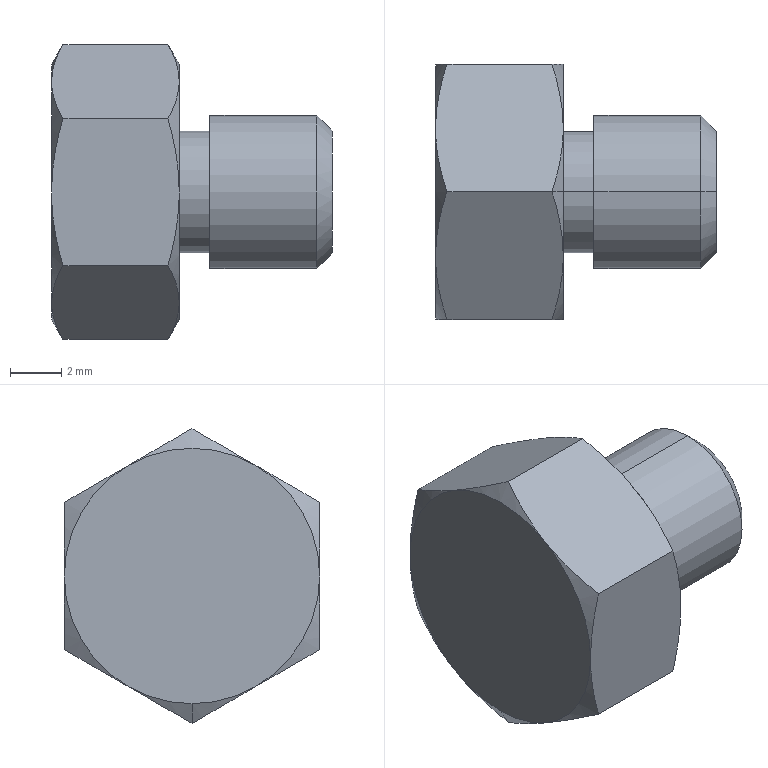Part | STEP file | 11-STEHN1011 | 1 solid | 30 faces | box 11 x 10 x 11.547 mm | volume 584.701 mm3 | cone 16 | plane 10 | cylinder 4 | commonest cylinder face diameters 4.773 x2 6 x2
STEP:
#1=CARTESIAN_POINT('',(5.386,0.,3.));
#2=VERTEX_POINT('',#1);
#3=CARTESIAN_POINT('',(5.386,0.,-3.));
#4=VERTEX_POINT('',#3);
#5=CARTESIAN_POINT('',(5.386,0.,0.));
#6=DIRECTION('',(-1.,0.,0.));
#7=DIRECTION('',(0.,0.,1.));
#8=AXIS2_PLACEMENT_3D('',#5,#6,#7);
#9=CIRCLE('',#8,3.);
#10=EDGE_CURVE('',#2,#4,#9,.T.);
#11=ORIENTED_EDGE('',*,*,#10,.T.);
#12=CARTESIAN_POINT('',(1.2,0.,-3.));
#13=VERTEX_POINT('',#12);
#14=CARTESIAN_POINT('',(5.386,0.,-3.));
#15=DIRECTION('',(-1.,0.,0.));
#16=VECTOR('',#15,1000.);
#17=LINE('',#14,#16);
#18=EDGE_CURVE('',#4,#13,#17,.T.);
#19=ORIENTED_EDGE('',*,*,#18,.T.);
#20=CARTESIAN_POINT('',(1.2,0.,3.));
#21=VERTEX_POINT('',#20);
#22=CARTESIAN_POINT('',(1.2,0.,0.));
#23=DIRECTION('',(1.,0.,0.));
#24=DIRECTION('',(0.,0.,1.));
#25=AXIS2_PLACEMENT_3D('',#22,#23,#24);
#26=CIRCLE('',#25,3.);
#27=EDGE_CURVE('',#13,#21,#26,.T.);
#28=ORIENTED_EDGE('',*,*,#27,.T.);
#29=CARTESIAN_POINT('',(5.386,0.,3.));
#30=DIRECTION('',(-1.,0.,0.));
#31=VECTOR('',#30,1000.);
#32=LINE('',#29,#31);
#33=EDGE_CURVE('',#2,#21,#32,.T.);
#34=ORIENTED_EDGE('',*,*,#33,.F.);
#35=EDGE_LOOP('',(#11,#19,#28,#34));
#36=FACE_OUTER_BOUND('',#35,.T.);
#37=CARTESIAN_POINT('',(5.386,0.,0.));
#38=DIRECTION('',(-1.,0.,0.));
#39=DIRECTION('',(0.,0.,1.));
#40=AXIS2_PLACEMENT_3D('',#37,#38,#39);
#41=CYLINDRICAL_SURFACE('',#40,3.);
#42=ADVANCED_FACE('',(#36),#41,.T.);
#43=CARTESIAN_POINT('',(6.,0.,2.386));
#44=VERTEX_POINT('',#43);
#45=CARTESIAN_POINT('',(6.,0.,-2.386));
#46=VERTEX_POINT('',#45);
#47=CARTESIAN_POINT('',(6.,0.,0.));
#48=DIRECTION('',(-1.,0.,0.));
#49=DIRECTION('',(0.,0.,1.));
#50=AXIS2_PLACEMENT_3D('',#47,#48,#49);
#51=CIRCLE('',#50,2.386);
#52=EDGE_CURVE('',#44,#46,#51,.T.);
#53=ORIENTED_EDGE('',*,*,#52,.T.);
#54=CARTESIAN_POINT('',(6.,0.,-2.386));
#55=DIRECTION('',(-0.7071,0.,-0.7071));
#56=VECTOR('',#55,1000.);
#57=LINE('',#54,#56);
#58=EDGE_CURVE('',#46,#4,#57,.T.);
#59=ORIENTED_EDGE('',*,*,#58,.T.);
#60=ORIENTED_EDGE('',*,*,#10,.F.);
#61=CARTESIAN_POINT('',(6.,0.,2.386));
#62=DIRECTION('',(-0.7071,0.,0.7071));
#63=VECTOR('',#62,1000.);
#64=LINE('',#61,#63);
#65=EDGE_CURVE('',#44,#2,#64,.T.);
#66=ORIENTED_EDGE('',*,*,#65,.F.);
#67=EDGE_LOOP('',(#53,#59,#60,#66));
#68=FACE_OUTER_BOUND('',#67,.T.);
#69=CARTESIAN_POINT('',(6.,0.,0.));
#70=DIRECTION('',(-1.,0.,0.));
#71=DIRECTION('',(0.,0.,1.));
#72=AXIS2_PLACEMENT_3D('',#69,#70,#71);
#73=CONICAL_SURFACE('',#72,2.386,0.7854);
#74=ADVANCED_FACE('',(#68),#73,.T.);
#75=CARTESIAN_POINT('',(0.,0.,-2.387));
#76=VERTEX_POINT('',#75);
#77=CARTESIAN_POINT('',(0.,0.,2.387));
#78=VERTEX_POINT('',#77);
#79=CARTESIAN_POINT('',(0.,0.,0.));
#80=DIRECTION('',(1.,0.,0.));
#81=DIRECTION('',(0.,0.,-1.));
#82=AXIS2_PLACEMENT_3D('',#79,#80,#81);
#83=CIRCLE('',#82,2.387);
#84=EDGE_CURVE('',#76,#78,#83,.T.);
#85=ORIENTED_EDGE('',*,*,#84,.T.);
#86=CARTESIAN_POINT('',(1.2,0.,2.387));
#87=VERTEX_POINT('',#86);
#88=CARTESIAN_POINT('',(0.,0.,2.387));
#89=DIRECTION('',(1.,0.,0.));
#90=VECTOR('',#89,1000.);
#91=LINE('',#88,#90);
#92=EDGE_CURVE('',#78,#87,#91,.T.);
#93=ORIENTED_EDGE('',*,*,#92,.T.);
#94=CARTESIAN_POINT('',(1.2,0.,-2.387));
#95=VERTEX_POINT('',#94);
#96=CARTESIAN_POINT('',(1.2,0.,0.));
#97=DIRECTION('',(1.,0.,0.));
#98=DIRECTION('',(0.,0.,-1.));
#99=AXIS2_PLACEMENT_3D('',#96,#97,#98);
#100=CIRCLE('',#99,2.387);
#101=EDGE_CURVE('',#95,#87,#100,.T.);
#102=ORIENTED_EDGE('',*,*,#101,.F.);
#103=CARTESIAN_POINT('',(0.,0.,-2.387));
#104=DIRECTION('',(1.,0.,0.));
#105=VECTOR('',#104,1000.);
#106=LINE('',#103,#105);
#107=EDGE_CURVE('',#76,#95,#106,.T.);
#108=ORIENTED_EDGE('',*,*,#107,.F.);
#109=EDGE_LOOP('',(#85,#93,#102,#108));
#110=FACE_OUTER_BOUND('',#109,.T.);
#111=CARTESIAN_POINT('',(0.,0.,0.));
#112=DIRECTION('',(1.,0.,0.));
#113=DIRECTION('',(0.,0.,-1.));
#114=AXIS2_PLACEMENT_3D('',#111,#112,#113);
#115=CYLINDRICAL_SURFACE('',#114,2.387);
#116=ADVANCED_FACE('',(#110),#115,.T.);
#117=CARTESIAN_POINT('',(0.,0.,5.));
#118=VERTEX_POINT('',#117);
#119=CARTESIAN_POINT('',(0.,-2.5,4.33));
#120=VERTEX_POINT('',#119);
#121=CARTESIAN_POINT('',(0.,0.,0.));
#122=DIRECTION('',(1.,0.,0.));
#123=DIRECTION('',(0.,0.,1.));
#124=AXIS2_PLACEMENT_3D('',#121,#122,#123);
#125=CIRCLE('',#124,5.);
#126=EDGE_CURVE('',#118,#120,#125,.T.);
#127=ORIENTED_EDGE('',*,*,#126,.F.);
#128=CARTESIAN_POINT('',(-0.4466,0.,5.774));
#129=VERTEX_POINT('',#128);
#130=CARTESIAN_POINT('',(0.,0.,5.));
#131=DIRECTION('',(-0.5,0.,0.866));
#132=VECTOR('',#131,1000.);
#133=LINE('',#130,#132);
#134=EDGE_CURVE('',#118,#129,#133,.T.);
#135=ORIENTED_EDGE('',*,*,#134,.T.);
#136=CARTESIAN_POINT('',(-0.4466,0.,5.774));
#137=CARTESIAN_POINT('',(-0.1743,-0.8168,5.302));
#138=CARTESIAN_POINT('',(0.,-1.647,4.823));
#139=CARTESIAN_POINT('',(0.,-2.5,4.33));
#140=B_SPLINE_CURVE_WITH_KNOTS('',3,(#136,#137,#138,#139),.UNSPECIFIED.,.F.,.F.,(4,4),(0.,0.002921),.UNSPECIFIED.);
#141=EDGE_CURVE('',#129,#120,#140,.T.);
#142=ORIENTED_EDGE('',*,*,#141,.T.);
#143=EDGE_LOOP('',(#127,#135,#142));
#144=FACE_OUTER_BOUND('',#143,.T.);
#145=CARTESIAN_POINT('',(0.,0.,0.));
#146=DIRECTION('',(-1.,0.,0.));
#147=DIRECTION('',(0.,0.,1.));
#148=AXIS2_PLACEMENT_3D('',#145,#146,#147);
#149=CONICAL_SURFACE('',#148,5.,1.047);
#150=ADVANCED_FACE('',(#144),#149,.T.);
#151=CARTESIAN_POINT('',(-5.,-2.5,-4.33));
#152=VERTEX_POINT('',#151);
#153=CARTESIAN_POINT('',(-5.,0.,-5.));
#154=VERTEX_POINT('',#153);
#155=CARTESIAN_POINT('',(-5.,0.,0.));
#156=DIRECTION('',(1.,0.,0.));
#157=DIRECTION('',(0.,0.,-1.));
#158=AXIS2_PLACEMENT_3D('',#155,#156,#157);
#159=CIRCLE('',#158,5.);
#160=EDGE_CURVE('',#152,#154,#159,.T.);
#161=ORIENTED_EDGE('',*,*,#160,.T.);
#162=CARTESIAN_POINT('',(-4.553,0.,-5.774));
#163=VERTEX_POINT('',#162);
#164=CARTESIAN_POINT('',(-5.,0.,-5.));
#165=DIRECTION('',(0.5,0.,-0.866));
#166=VECTOR('',#165,1000.);
#167=LINE('',#164,#166);
#168=EDGE_CURVE('',#154,#163,#167,.T.);
#169=ORIENTED_EDGE('',*,*,#168,.T.);
#170=CARTESIAN_POINT('',(-5.,-2.5,-4.33));
#171=CARTESIAN_POINT('',(-5.,-2.076,-4.575));
#172=CARTESIAN_POINT('',(-4.958,-1.654,-4.818));
#173=CARTESIAN_POINT('',(-4.802,-0.8183,-5.301));
#174=CARTESIAN_POINT('',(-4.689,-0.4069,-5.539));
#175=CARTESIAN_POINT('',(-4.553,0.,-5.774));
#176=B_SPLINE_CURVE_WITH_KNOTS('',3,(#170,#171,#172,#173,#174,#175),.UNSPECIFIED.,.F.,.F.,(4,2,4),(0.,0.001464,0.002928),.UNSPECIFIED.);
#177=EDGE_CURVE('',#152,#163,#176,.T.);
#178=ORIENTED_EDGE('',*,*,#177,.F.);
#179=EDGE_LOOP('',(#161,#169,#178));
#180=FACE_OUTER_BOUND('',#179,.T.);
#181=CARTESIAN_POINT('',(-5.,0.,0.));
#182=DIRECTION('',(1.,0.,0.));
#183=DIRECTION('',(0.,0.,-1.));
#184=AXIS2_PLACEMENT_3D('',#181,#182,#183);
#185=CONICAL_SURFACE('',#184,5.,1.047);
#186=ADVANCED_FACE('',(#180),#185,.T.);
#187=ORIENTED_EDGE('',*,*,#18,.F.);
#188=CARTESIAN_POINT('',(5.386,0.,0.));
#189=DIRECTION('',(-1.,0.,0.));
#190=DIRECTION('',(0.,0.,1.));
#191=AXIS2_PLACEMENT_3D('',#188,#189,#190);
#192=CIRCLE('',#191,3.);
#193=EDGE_CURVE('',#4,#2,#192,.T.);
#194=ORIENTED_EDGE('',*,*,#193,.T.);
#195=ORIENTED_EDGE('',*,*,#33,.T.);
#196=CARTESIAN_POINT('',(1.2,0.,0.));
#197=DIRECTION('',(1.,0.,0.));
#198=DIRECTION('',(0.,0.,1.));
#199=AXIS2_PLACEMENT_3D('',#196,#197,#198);
#200=CIRCLE('',#199,3.);
#201=EDGE_CURVE('',#21,#13,#200,.T.);
#202=ORIENTED_EDGE('',*,*,#201,.T.);
#203=EDGE_LOOP('',(#187,#194,#195,#202));
#204=FACE_OUTER_BOUND('',#203,.T.);
#205=CARTESIAN_POINT('',(5.386,0.,0.));
#206=DIRECTION('',(-1.,0.,0.));
#207=DIRECTION('',(0.,0.,1.));
#208=AXIS2_PLACEMENT_3D('',#205,#206,#207);
#209=CYLINDRICAL_SURFACE('',#208,3.);
#210=ADVANCED_FACE('',(#204),#209,.T.);
#211=ORIENTED_EDGE('',*,*,#58,.F.);
#212=CARTESIAN_POINT('',(6.,0.,0.));
#213=DIRECTION('',(-1.,0.,0.));
#214=DIRECTION('',(0.,0.,1.));
#215=AXIS2_PLACEMENT_3D('',#212,#213,#214);
#216=CIRCLE('',#215,2.386);
#217=EDGE_CURVE('',#46,#44,#216,.T.);
#218=ORIENTED_EDGE('',*,*,#217,.T.);
#219=ORIENTED_EDGE('',*,*,#65,.T.);
#220=ORIENTED_EDGE('',*,*,#193,.F.);
#221=EDGE_LOOP('',(#211,#218,#219,#220));
#222=FACE_OUTER_BOUND('',#221,.T.);
#223=CARTESIAN_POINT('',(6.,0.,0.));
#224=DIRECTION('',(-1.,0.,0.));
#225=DIRECTION('',(0.,0.,1.));
#226=AXIS2_PLACEMENT_3D('',#223,#224,#225);
#227=CONICAL_SURFACE('',#226,2.386,0.7854);
#228=ADVANCED_FACE('',(#222),#227,.T.);
#229=ORIENTED_EDGE('',*,*,#101,.T.);
#230=CARTESIAN_POINT('',(1.2,0.,0.));
#231=DIRECTION('',(1.,0.,0.));
#232=DIRECTION('',(0.,0.,-1.));
#233=AXIS2_PLACEMENT_3D('',#230,#231,#232);
#234=CIRCLE('',#233,2.387);
#235=EDGE_CURVE('',#87,#95,#234,.T.);
#236=ORIENTED_EDGE('',*,*,#235,.T.);
#237=EDGE_LOOP('',(#229,#236));
#238=FACE_BOUND('',#237,.T.);
#239=ORIENTED_EDGE('',*,*,#201,.F.);
#240=ORIENTED_EDGE('',*,*,#27,.F.);
#241=EDGE_LOOP('',(#239,#240));
#242=FACE_OUTER_BOUND('',#241,.T.);
#243=CARTESIAN_POINT('',(1.2,3.,3.));
#244=DIRECTION('',(-1.,0.,0.));
#245=DIRECTION('',(0.,0.,-1.));
#246=AXIS2_PLACEMENT_3D('',#243,#244,#245);
#247=PLANE('',#246);
#248=ADVANCED_FACE('',(#238,#242),#247,.T.);
#249=ORIENTED_EDGE('',*,*,#52,.F.);
#250=ORIENTED_EDGE('',*,*,#217,.F.);
#251=EDGE_LOOP('',(#249,#250));
#252=FACE_OUTER_BOUND('',#251,.T.);
#253=CARTESIAN_POINT('',(6.,2.386,-2.386));
#254=DIRECTION('',(1.,0.,0.));
#255=DIRECTION('',(0.,0.,1.));
#256=AXIS2_PLACEMENT_3D('',#253,#254,#255);
#257=PLANE('',#256);
#258=ADVANCED_FACE('',(#252),#257,.T.);
#259=ORIENTED_EDGE('',*,*,#92,.F.);
#260=CARTESIAN_POINT('',(0.,0.,0.));
#261=DIRECTION('',(1.,0.,0.));
#262=DIRECTION('',(0.,0.,-1.));
#263=AXIS2_PLACEMENT_3D('',#260,#261,#262);
#264=CIRCLE('',#263,2.387);
#265=EDGE_CURVE('',#78,#76,#264,.T.);
#266=ORIENTED_EDGE('',*,*,#265,.T.);
#267=ORIENTED_EDGE('',*,*,#107,.T.);
#268=ORIENTED_EDGE('',*,*,#235,.F.);
#269=EDGE_LOOP('',(#259,#266,#267,#268));
#270=FACE_OUTER_BOUND('',#269,.T.);
#271=CARTESIAN_POINT('',(0.,0.,0.));
#272=DIRECTION('',(1.,0.,0.));
#273=DIRECTION('',(0.,0.,-1.));
#274=AXIS2_PLACEMENT_3D('',#271,#272,#273);
#275=CYLINDRICAL_SURFACE('',#274,2.387);
#276=ADVANCED_FACE('',(#270),#275,.T.);
#277=ORIENTED_EDGE('',*,*,#84,.F.);
#278=ORIENTED_EDGE('',*,*,#265,.F.);
#279=EDGE_LOOP('',(#277,#278));
#280=FACE_BOUND('',#279,.T.);
#281=CARTESIAN_POINT('',(0.,-5.,0.));
#282=VERTEX_POINT('',#281);
#283=CARTESIAN_POINT('',(0.,0.,0.));
#284=DIRECTION('',(1.,0.,0.));
#285=DIRECTION('',(0.,0.,1.));
#286=AXIS2_PLACEMENT_3D('',#283,#284,#285);
#287=CIRCLE('',#286,5.);
#288=EDGE_CURVE('',#120,#282,#287,.T.);
#289=ORIENTED_EDGE('',*,*,#288,.T.);
#290=CARTESIAN_POINT('',(0.,-2.5,-4.33));
#291=VERTEX_POINT('',#290);
#292=CARTESIAN_POINT('',(0.,0.,0.));
#293=DIRECTION('',(1.,0.,0.));
#294=DIRECTION('',(0.,0.,1.));
#295=AXIS2_PLACEMENT_3D('',#292,#293,#294);
#296=CIRCLE('',#295,5.);
#297=EDGE_CURVE('',#282,#291,#296,.T.);
#298=ORIENTED_EDGE('',*,*,#297,.T.);
#299=CARTESIAN_POINT('',(0.,2.5,-4.33));
#300=VERTEX_POINT('',#299);
#301=CARTESIAN_POINT('',(0.,0.,0.));
#302=DIRECTION('',(1.,0.,0.));
#303=DIRECTION('',(0.,0.,1.));
#304=AXIS2_PLACEMENT_3D('',#301,#302,#303);
#305=CIRCLE('',#304,5.);
#306=EDGE_CURVE('',#291,#300,#305,.T.);
#307=ORIENTED_EDGE('',*,*,#306,.T.);
#308=CARTESIAN_POINT('',(0.,5.,0.));
#309=VERTEX_POINT('',#308);
#310=CARTESIAN_POINT('',(0.,0.,0.));
#311=DIRECTION('',(1.,0.,0.));
#312=DIRECTION('',(0.,0.,1.));
#313=AXIS2_PLACEMENT_3D('',#310,#311,#312);
#314=CIRCLE('',#313,5.);
#315=EDGE_CURVE('',#300,#309,#314,.T.);
#316=ORIENTED_EDGE('',*,*,#315,.T.);
#317=CARTESIAN_POINT('',(0.,2.5,4.33));
#318=VERTEX_POINT('',#317);
#319=CARTESIAN_POINT('',(0.,0.,0.));
#320=DIRECTION('',(1.,0.,0.));
#321=DIRECTION('',(0.,0.,1.));
#322=AXIS2_PLACEMENT_3D('',#319,#320,#321);
#323=CIRCLE('',#322,5.);
#324=EDGE_CURVE('',#309,#318,#323,.T.);
#325=ORIENTED_EDGE('',*,*,#324,.T.);
#326=CARTESIAN_POINT('',(0.,0.,0.));
#327=DIRECTION('',(1.,0.,0.));
#328=DIRECTION('',(0.,0.,1.));
#329=AXIS2_PLACEMENT_3D('',#326,#327,#328);
#330=CIRCLE('',#329,5.);
#331=EDGE_CURVE('',#318,#118,#330,.T.);
#332=ORIENTED_EDGE('',*,*,#331,.T.);
#333=ORIENTED_EDGE('',*,*,#126,.T.);
#334=EDGE_LOOP('',(#289,#298,#307,#316,#325,#332,#333));
#335=FACE_OUTER_BOUND('',#334,.T.);
#336=CARTESIAN_POINT('',(0.,-5.,5.));
#337=DIRECTION('',(1.,0.,0.));
#338=DIRECTION('',(0.,0.,-1.));
#339=AXIS2_PLACEMENT_3D('',#336,#337,#338);
#340=PLANE('',#339);
#341=ADVANCED_FACE('',(#280,#335),#340,.T.);
#342=CARTESIAN_POINT('',(-0.4466,-5.,-2.887));
#343=VERTEX_POINT('',#342);
#344=CARTESIAN_POINT('',(-0.4466,-5.,-2.887));
#345=CARTESIAN_POINT('',(-0.1743,-4.183,-3.358));
#346=CARTESIAN_POINT('',(0.,-3.353,-3.837));
#347=CARTESIAN_POINT('',(0.,-2.5,-4.33));
#348=B_SPLINE_CURVE_WITH_KNOTS('',3,(#344,#345,#346,#347),.UNSPECIFIED.,.F.,.F.,(4,4),(0.,0.002921),.UNSPECIFIED.);
#349=EDGE_CURVE('',#343,#291,#348,.T.);
#350=ORIENTED_EDGE('',*,*,#349,.T.);
#351=ORIENTED_EDGE('',*,*,#297,.F.);
#352=CARTESIAN_POINT('',(0.,-5.,0.));
#353=CARTESIAN_POINT('',(0.,-5.,-0.9853));
#354=CARTESIAN_POINT('',(-0.1743,-5.,-1.944));
#355=CARTESIAN_POINT('',(-0.4466,-5.,-2.887));
#356=B_SPLINE_CURVE_WITH_KNOTS('',3,(#352,#353,#354,#355),.UNSPECIFIED.,.F.,.F.,(4,4),(0.,0.002921),.UNSPECIFIED.);
#357=EDGE_CURVE('',#282,#343,#356,.T.);
#358=ORIENTED_EDGE('',*,*,#357,.T.);
#359=EDGE_LOOP('',(#350,#351,#358));
#360=FACE_OUTER_BOUND('',#359,.T.);
#361=CARTESIAN_POINT('',(0.,0.,0.));
#362=DIRECTION('',(-1.,0.,0.));
#363=DIRECTION('',(0.,0.,1.));
#364=AXIS2_PLACEMENT_3D('',#361,#362,#363);
#365=CONICAL_SURFACE('',#364,5.,1.047);
#366=ADVANCED_FACE('',(#360),#365,.T.);
#367=CARTESIAN_POINT('',(-0.4466,-5.,2.887));
#368=VERTEX_POINT('',#367);
#369=CARTESIAN_POINT('',(-0.4466,-5.,2.887));
#370=CARTESIAN_POINT('',(-0.3109,-5.,2.417));
#371=CARTESIAN_POINT('',(-0.1985,-5.,1.942));
#372=CARTESIAN_POINT('',(-0.04234,-5.,0.9764));
#373=CARTESIAN_POINT('',(0.,-5.,0.4895));
#374=CARTESIAN_POINT('',(0.,-5.,0.));
#375=B_SPLINE_CURVE_WITH_KNOTS('',3,(#369,#370,#371,#372,#373,#374),.UNSPECIFIED.,.F.,.F.,(4,2,4),(-0.00158,-0.0001154,0.001349),.UNSPECIFIED.);
#376=EDGE_CURVE('',#368,#282,#375,.T.);
#377=ORIENTED_EDGE('',*,*,#376,.T.);
#378=ORIENTED_EDGE('',*,*,#288,.F.);
#379=CARTESIAN_POINT('',(0.,-2.5,4.33));
#380=CARTESIAN_POINT('',(0.,-3.353,3.837));
#381=CARTESIAN_POINT('',(-0.1743,-4.183,3.358));
#382=CARTESIAN_POINT('',(-0.4466,-5.,2.887));
#383=B_SPLINE_CURVE_WITH_KNOTS('',3,(#379,#380,#381,#382),.UNSPECIFIED.,.F.,.F.,(4,4),(0.,0.002921),.UNSPECIFIED.);
#384=EDGE_CURVE('',#120,#368,#383,.T.);
#385=ORIENTED_EDGE('',*,*,#384,.T.);
#386=EDGE_LOOP('',(#377,#378,#385));
#387=FACE_OUTER_BOUND('',#386,.T.);
#388=CARTESIAN_POINT('',(0.,0.,0.));
#389=DIRECTION('',(-1.,0.,0.));
#390=DIRECTION('',(0.,0.,1.));
#391=AXIS2_PLACEMENT_3D('',#388,#389,#390);
#392=CONICAL_SURFACE('',#391,5.,1.047);
#393=ADVANCED_FACE('',(#387),#392,.T.);
#394=ORIENTED_EDGE('',*,*,#134,.F.);
#395=ORIENTED_EDGE('',*,*,#331,.F.);
#396=CARTESIAN_POINT('',(0.,2.5,4.33));
#397=CARTESIAN_POINT('',(0.,1.647,4.823));
#398=CARTESIAN_POINT('',(-0.1743,0.8168,5.302));
#399=CARTESIAN_POINT('',(-0.4466,0.,5.774));
#400=B_SPLINE_CURVE_WITH_KNOTS('',3,(#396,#397,#398,#399),.UNSPECIFIED.,.F.,.F.,(4,4),(0.,0.002921),.UNSPECIFIED.);
#401=EDGE_CURVE('',#318,#129,#400,.T.);
#402=ORIENTED_EDGE('',*,*,#401,.T.);
#403=EDGE_LOOP('',(#394,#395,#402));
#404=FACE_OUTER_BOUND('',#403,.T.);
#405=CARTESIAN_POINT('',(0.,0.,0.));
#406=DIRECTION('',(-1.,0.,0.));
#407=DIRECTION('',(0.,0.,1.));
#408=AXIS2_PLACEMENT_3D('',#405,#406,#407);
#409=CONICAL_SURFACE('',#408,5.,1.047);
#410=ADVANCED_FACE('',(#404),#409,.T.);
#411=ORIENTED_EDGE('',*,*,#324,.F.);
#412=CARTESIAN_POINT('',(-0.4466,5.,2.887));
#413=VERTEX_POINT('',#412);
#414=CARTESIAN_POINT('',(0.,5.,0.));
#415=CARTESIAN_POINT('',(0.,5.,0.9853));
#416=CARTESIAN_POINT('',(-0.1743,5.,1.944));
#417=CARTESIAN_POINT('',(-0.4466,5.,2.887));
#418=B_SPLINE_CURVE_WITH_KNOTS('',3,(#414,#415,#416,#417),.UNSPECIFIED.,.F.,.F.,(4,4),(0.,0.002921),.UNSPECIFIED.);
#419=EDGE_CURVE('',#309,#413,#418,.T.);
#420=ORIENTED_EDGE('',*,*,#419,.T.);
#421=CARTESIAN_POINT('',(-0.4466,5.,2.887));
#422=CARTESIAN_POINT('',(-0.1743,4.183,3.358));
#423=CARTESIAN_POINT('',(0.,3.353,3.837));
#424=CARTESIAN_POINT('',(0.,2.5,4.33));
#425=B_SPLINE_CURVE_WITH_KNOTS('',3,(#421,#422,#423,#424),.UNSPECIFIED.,.F.,.F.,(4,4),(0.,0.002921),.UNSPECIFIED.);
#426=EDGE_CURVE('',#413,#318,#425,.T.);
#427=ORIENTED_EDGE('',*,*,#426,.T.);
#428=EDGE_LOOP('',(#411,#420,#427));
#429=FACE_OUTER_BOUND('',#428,.T.);
#430=CARTESIAN_POINT('',(0.,0.,0.));
#431=DIRECTION('',(-1.,0.,0.));
#432=DIRECTION('',(0.,0.,1.));
#433=AXIS2_PLACEMENT_3D('',#430,#431,#432);
#434=CONICAL_SURFACE('',#433,5.,1.047);
#435=ADVANCED_FACE('',(#429),#434,.T.);
#436=CARTESIAN_POINT('',(-0.4466,5.,-2.887));
#437=VERTEX_POINT('',#436);
#438=CARTESIAN_POINT('',(-0.4466,5.,-2.887));
#439=CARTESIAN_POINT('',(-0.3109,5.,-2.417));
#440=CARTESIAN_POINT('',(-0.1985,5.,-1.942));
#441=CARTESIAN_POINT('',(-0.04234,5.,-0.9764));
#442=CARTESIAN_POINT('',(0.,5.,-0.4895));
#443=CARTESIAN_POINT('',(0.,5.,0.));
#444=B_SPLINE_CURVE_WITH_KNOTS('',3,(#438,#439,#440,#441,#442,#443),.UNSPECIFIED.,.F.,.F.,(4,2,4),(-0.00158,-0.0001154,0.001349),.UNSPECIFIED.);
#445=EDGE_CURVE('',#437,#309,#444,.T.);
#446=ORIENTED_EDGE('',*,*,#445,.T.);
#447=ORIENTED_EDGE('',*,*,#315,.F.);
#448=CARTESIAN_POINT('',(0.,2.5,-4.33));
#449=CARTESIAN_POINT('',(0.,3.353,-3.837));
#450=CARTESIAN_POINT('',(-0.1743,4.183,-3.358));
#451=CARTESIAN_POINT('',(-0.4466,5.,-2.887));
#452=B_SPLINE_CURVE_WITH_KNOTS('',3,(#448,#449,#450,#451),.UNSPECIFIED.,.F.,.F.,(4,4),(0.,0.002921),.UNSPECIFIED.);
#453=EDGE_CURVE('',#300,#437,#452,.T.);
#454=ORIENTED_EDGE('',*,*,#453,.T.);
#455=EDGE_LOOP('',(#446,#447,#454));
#456=FACE_OUTER_BOUND('',#455,.T.);
#457=CARTESIAN_POINT('',(0.,0.,0.));
#458=DIRECTION('',(-1.,0.,0.));
#459=DIRECTION('',(0.,0.,1.));
#460=AXIS2_PLACEMENT_3D('',#457,#458,#459);
#461=CONICAL_SURFACE('',#460,5.,1.047);
#462=ADVANCED_FACE('',(#456),#461,.T.);
#463=ORIENTED_EDGE('',*,*,#306,.F.);
#464=CARTESIAN_POINT('',(-0.4466,0.,-5.774));
#465=VERTEX_POINT('',#464);
#466=CARTESIAN_POINT('',(0.,-2.5,-4.33));
#467=CARTESIAN_POINT('',(0.,-1.647,-4.823));
#468=CARTESIAN_POINT('',(-0.1743,-0.8168,-5.302));
#469=CARTESIAN_POINT('',(-0.4466,0.,-5.774));
#470=B_SPLINE_CURVE_WITH_KNOTS('',3,(#466,#467,#468,#469),.UNSPECIFIED.,.F.,.F.,(4,4),(0.,0.002921),.UNSPECIFIED.);
#471=EDGE_CURVE('',#291,#465,#470,.T.);
#472=ORIENTED_EDGE('',*,*,#471,.T.);
#473=CARTESIAN_POINT('',(-0.4466,0.,-5.774));
#474=CARTESIAN_POINT('',(-0.1743,0.8168,-5.302));
#475=CARTESIAN_POINT('',(0.,1.647,-4.823));
#476=CARTESIAN_POINT('',(0.,2.5,-4.33));
#477=B_SPLINE_CURVE_WITH_KNOTS('',3,(#473,#474,#475,#476),.UNSPECIFIED.,.F.,.F.,(4,4),(0.,0.002921),.UNSPECIFIED.);
#478=EDGE_CURVE('',#465,#300,#477,.T.);
#479=ORIENTED_EDGE('',*,*,#478,.T.);
#480=EDGE_LOOP('',(#463,#472,#479));
#481=FACE_OUTER_BOUND('',#480,.T.);
#482=CARTESIAN_POINT('',(0.,0.,0.));
#483=DIRECTION('',(-1.,0.,0.));
#484=DIRECTION('',(0.,0.,1.));
#485=AXIS2_PLACEMENT_3D('',#482,#483,#484);
#486=CONICAL_SURFACE('',#485,5.,1.047);
#487=ADVANCED_FACE('',(#481),#486,.T.);
#488=CARTESIAN_POINT('',(-2.5,0.,-5.774));
#489=DIRECTION('',(1.,0.,0.));
#490=VECTOR('',#489,1000.);
#491=LINE('',#488,#490);
#492=EDGE_CURVE('',#163,#465,#491,.T.);
#493=ORIENTED_EDGE('',*,*,#492,.T.);
#494=ORIENTED_EDGE('',*,*,#471,.F.);
#495=ORIENTED_EDGE('',*,*,#349,.F.);
#496=CARTESIAN_POINT('',(-4.553,-5.,-2.887));
#497=VERTEX_POINT('',#496);
#498=CARTESIAN_POINT('',(-2.5,-5.,-2.887));
#499=DIRECTION('',(-1.,0.,0.));
#500=VECTOR('',#499,1000.);
#501=LINE('',#498,#500);
#502=EDGE_CURVE('',#343,#497,#501,.T.);
#503=ORIENTED_EDGE('',*,*,#502,.T.);
#504=CARTESIAN_POINT('',(-4.553,-5.,-2.887));
#505=CARTESIAN_POINT('',(-4.826,-4.183,-3.358));
#506=CARTESIAN_POINT('',(-5.,-3.353,-3.837));
#507=CARTESIAN_POINT('',(-5.,-2.5,-4.33));
#508=B_SPLINE_CURVE_WITH_KNOTS('',3,(#504,#505,#506,#507),.UNSPECIFIED.,.F.,.F.,(4,4),(0.,0.002921),.UNSPECIFIED.);
#509=EDGE_CURVE('',#497,#152,#508,.T.);
#510=ORIENTED_EDGE('',*,*,#509,.T.);
#511=ORIENTED_EDGE('',*,*,#177,.T.);
#512=EDGE_LOOP('',(#493,#494,#495,#503,#510,#511));
#513=FACE_OUTER_BOUND('',#512,.T.);
#514=CARTESIAN_POINT('',(0.,-5.,-2.887));
#515=DIRECTION('',(0.,-0.5,-0.866));
#516=DIRECTION('',(-1.,0.,0.));
#517=AXIS2_PLACEMENT_3D('',#514,#515,#516);
#518=PLANE('',#517);
#519=ADVANCED_FACE('',(#513),#518,.T.);
#520=ORIENTED_EDGE('',*,*,#502,.F.);
#521=ORIENTED_EDGE('',*,*,#357,.F.);
#522=ORIENTED_EDGE('',*,*,#376,.F.);
#523=CARTESIAN_POINT('',(-4.553,-5.,2.887));
#524=VERTEX_POINT('',#523);
#525=CARTESIAN_POINT('',(-2.5,-5.,2.887));
#526=DIRECTION('',(-1.,0.,0.));
#527=VECTOR('',#526,1000.);
#528=LINE('',#525,#527);
#529=EDGE_CURVE('',#368,#524,#528,.T.);
#530=ORIENTED_EDGE('',*,*,#529,.T.);
#531=CARTESIAN_POINT('',(-5.,-5.,0.));
#532=VERTEX_POINT('',#531);
#533=CARTESIAN_POINT('',(-4.553,-5.,2.887));
#534=CARTESIAN_POINT('',(-4.826,-5.,1.944));
#535=CARTESIAN_POINT('',(-5.,-5.,0.9853));
#536=CARTESIAN_POINT('',(-5.,-5.,0.));
#537=B_SPLINE_CURVE_WITH_KNOTS('',3,(#533,#534,#535,#536),.UNSPECIFIED.,.F.,.F.,(4,4),(0.,0.002921),.UNSPECIFIED.);
#538=EDGE_CURVE('',#524,#532,#537,.T.);
#539=ORIENTED_EDGE('',*,*,#538,.T.);
#540=CARTESIAN_POINT('',(-5.,-5.,0.));
#541=CARTESIAN_POINT('',(-5.,-5.,-0.9853));
#542=CARTESIAN_POINT('',(-4.826,-5.,-1.944));
#543=CARTESIAN_POINT('',(-4.553,-5.,-2.887));
#544=B_SPLINE_CURVE_WITH_KNOTS('',3,(#540,#541,#542,#543),.UNSPECIFIED.,.F.,.F.,(4,4),(0.,0.002921),.UNSPECIFIED.);
#545=EDGE_CURVE('',#532,#497,#544,.T.);
#546=ORIENTED_EDGE('',*,*,#545,.T.);
#547=EDGE_LOOP('',(#520,#521,#522,#530,#539,#546));
#548=FACE_OUTER_BOUND('',#547,.T.);
#549=CARTESIAN_POINT('',(-5.,-5.,-2.887));
#550=DIRECTION('',(0.,-1.,0.));
#551=DIRECTION('',(1.,0.,0.));
#552=AXIS2_PLACEMENT_3D('',#549,#550,#551);
#553=PLANE('',#552);
#554=ADVANCED_FACE('',(#548),#553,.T.);
#555=ORIENTED_EDGE('',*,*,#529,.F.);
#556=ORIENTED_EDGE('',*,*,#384,.F.);
#557=ORIENTED_EDGE('',*,*,#141,.F.);
#558=CARTESIAN_POINT('',(-4.553,0.,5.774));
#559=VERTEX_POINT('',#558);
#560=CARTESIAN_POINT('',(-2.5,0.,5.774));
#561=DIRECTION('',(-1.,0.,0.));
#562=VECTOR('',#561,1000.);
#563=LINE('',#560,#562);
#564=EDGE_CURVE('',#129,#559,#563,.T.);
#565=ORIENTED_EDGE('',*,*,#564,.T.);
#566=CARTESIAN_POINT('',(-5.,-2.5,4.33));
#567=VERTEX_POINT('',#566);
#568=CARTESIAN_POINT('',(-4.553,0.,5.774));
#569=CARTESIAN_POINT('',(-4.826,-0.8168,5.302));
#570=CARTESIAN_POINT('',(-5.,-1.647,4.823));
#571=CARTESIAN_POINT('',(-5.,-2.5,4.33));
#572=B_SPLINE_CURVE_WITH_KNOTS('',3,(#568,#569,#570,#571),.UNSPECIFIED.,.F.,.F.,(4,4),(0.,0.002921),.UNSPECIFIED.);
#573=EDGE_CURVE('',#559,#567,#572,.T.);
#574=ORIENTED_EDGE('',*,*,#573,.T.);
#575=CARTESIAN_POINT('',(-5.,-2.5,4.33));
#576=CARTESIAN_POINT('',(-5.,-3.353,3.837));
#577=CARTESIAN_POINT('',(-4.826,-4.183,3.358));
#578=CARTESIAN_POINT('',(-4.553,-5.,2.887));
#579=B_SPLINE_CURVE_WITH_KNOTS('',3,(#575,#576,#577,#578),.UNSPECIFIED.,.F.,.F.,(4,4),(0.,0.002921),.UNSPECIFIED.);
#580=EDGE_CURVE('',#567,#524,#579,.T.);
#581=ORIENTED_EDGE('',*,*,#580,.T.);
#582=EDGE_LOOP('',(#555,#556,#557,#565,#574,#581));
#583=FACE_OUTER_BOUND('',#582,.T.);
#584=CARTESIAN_POINT('',(-5.,-5.,2.887));
#585=DIRECTION('',(0.,-0.5,0.866));
#586=DIRECTION('',(1.,0.,0.));
#587=AXIS2_PLACEMENT_3D('',#584,#585,#586);
#588=PLANE('',#587);
#589=ADVANCED_FACE('',(#583),#588,.T.);
#590=CARTESIAN_POINT('',(-5.,2.5,4.33));
#591=VERTEX_POINT('',#590);
#592=CARTESIAN_POINT('',(-5.,2.5,4.33));
#593=CARTESIAN_POINT('',(-5.,2.076,4.575));
#594=CARTESIAN_POINT('',(-4.958,1.654,4.818));
#595=CARTESIAN_POINT('',(-4.802,0.8183,5.301));
#596=CARTESIAN_POINT('',(-4.689,0.4069,5.539));
#597=CARTESIAN_POINT('',(-4.553,0.,5.774));
#598=B_SPLINE_CURVE_WITH_KNOTS('',3,(#592,#593,#594,#595,#596,#597),.UNSPECIFIED.,.F.,.F.,(4,2,4),(-0.001349,0.0001154,0.00158),.UNSPECIFIED.);
#599=EDGE_CURVE('',#591,#559,#598,.T.);
#600=ORIENTED_EDGE('',*,*,#599,.T.);
#601=ORIENTED_EDGE('',*,*,#564,.F.);
#602=ORIENTED_EDGE('',*,*,#401,.F.);
#603=ORIENTED_EDGE('',*,*,#426,.F.);
#604=CARTESIAN_POINT('',(-4.553,5.,2.887));
#605=VERTEX_POINT('',#604);
#606=CARTESIAN_POINT('',(-2.5,5.,2.887));
#607=DIRECTION('',(-1.,0.,0.));
#608=VECTOR('',#607,1000.);
#609=LINE('',#606,#608);
#610=EDGE_CURVE('',#413,#605,#609,.T.);
#611=ORIENTED_EDGE('',*,*,#610,.T.);
#612=CARTESIAN_POINT('',(-4.553,5.,2.887));
#613=CARTESIAN_POINT('',(-4.826,4.183,3.358));
#614=CARTESIAN_POINT('',(-5.,3.353,3.837));
#615=CARTESIAN_POINT('',(-5.,2.5,4.33));
#616=B_SPLINE_CURVE_WITH_KNOTS('',3,(#612,#613,#614,#615),.UNSPECIFIED.,.F.,.F.,(4,4),(0.,0.002921),.UNSPECIFIED.);
#617=EDGE_CURVE('',#605,#591,#616,.T.);
#618=ORIENTED_EDGE('',*,*,#617,.T.);
#619=EDGE_LOOP('',(#600,#601,#602,#603,#611,#618));
#620=FACE_OUTER_BOUND('',#619,.T.);
#621=CARTESIAN_POINT('',(-5.,0.,5.774));
#622=DIRECTION('',(0.,0.5,0.866));
#623=DIRECTION('',(1.,0.,0.));
#624=AXIS2_PLACEMENT_3D('',#621,#622,#623);
#625=PLANE('',#624);
#626=ADVANCED_FACE('',(#620),#625,.T.);
#627=CARTESIAN_POINT('',(-5.,5.,0.));
#628=VERTEX_POINT('',#627);
#629=CARTESIAN_POINT('',(-5.,5.,0.));
#630=CARTESIAN_POINT('',(-5.,5.,0.9853));
#631=CARTESIAN_POINT('',(-4.826,5.,1.944));
#632=CARTESIAN_POINT('',(-4.553,5.,2.887));
#633=B_SPLINE_CURVE_WITH_KNOTS('',3,(#629,#630,#631,#632),.UNSPECIFIED.,.F.,.F.,(4,4),(0.,0.002921),.UNSPECIFIED.);
#634=EDGE_CURVE('',#628,#605,#633,.T.);
#635=ORIENTED_EDGE('',*,*,#634,.T.);
#636=ORIENTED_EDGE('',*,*,#610,.F.);
#637=ORIENTED_EDGE('',*,*,#419,.F.);
#638=ORIENTED_EDGE('',*,*,#445,.F.);
#639=CARTESIAN_POINT('',(-4.553,5.,-2.887));
#640=VERTEX_POINT('',#639);
#641=CARTESIAN_POINT('',(-2.5,5.,-2.887));
#642=DIRECTION('',(-1.,0.,0.));
#643=VECTOR('',#642,1000.);
#644=LINE('',#641,#643);
#645=EDGE_CURVE('',#437,#640,#644,.T.);
#646=ORIENTED_EDGE('',*,*,#645,.T.);
#647=CARTESIAN_POINT('',(-4.553,5.,-2.887));
#648=CARTESIAN_POINT('',(-4.826,5.,-1.944));
#649=CARTESIAN_POINT('',(-5.,5.,-0.9853));
#650=CARTESIAN_POINT('',(-5.,5.,0.));
#651=B_SPLINE_CURVE_WITH_KNOTS('',3,(#647,#648,#649,#650),.UNSPECIFIED.,.F.,.F.,(4,4),(0.,0.002921),.UNSPECIFIED.);
#652=EDGE_CURVE('',#640,#628,#651,.T.);
#653=ORIENTED_EDGE('',*,*,#652,.T.);
#654=EDGE_LOOP('',(#635,#636,#637,#638,#646,#653));
#655=FACE_OUTER_BOUND('',#654,.T.);
#656=CARTESIAN_POINT('',(0.,5.,-2.887));
#657=DIRECTION('',(0.,1.,0.));
#658=DIRECTION('',(-1.,0.,0.));
#659=AXIS2_PLACEMENT_3D('',#656,#657,#658);
#660=PLANE('',#659);
#661=ADVANCED_FACE('',(#655),#660,.T.);
#662=CARTESIAN_POINT('',(-5.,2.5,-4.33));
#663=VERTEX_POINT('',#662);
#664=CARTESIAN_POINT('',(-5.,2.5,-4.33));
#665=CARTESIAN_POINT('',(-5.,3.353,-3.837));
#666=CARTESIAN_POINT('',(-4.826,4.183,-3.358));
#667=CARTESIAN_POINT('',(-4.553,5.,-2.887));
#668=B_SPLINE_CURVE_WITH_KNOTS('',3,(#664,#665,#666,#667),.UNSPECIFIED.,.F.,.F.,(4,4),(0.,0.002921),.UNSPECIFIED.);
#669=EDGE_CURVE('',#663,#640,#668,.T.);
#670=ORIENTED_EDGE('',*,*,#669,.T.);
#671=ORIENTED_EDGE('',*,*,#645,.F.);
#672=ORIENTED_EDGE('',*,*,#453,.F.);
#673=ORIENTED_EDGE('',*,*,#478,.F.);
#674=ORIENTED_EDGE('',*,*,#492,.F.);
#675=CARTESIAN_POINT('',(-4.553,0.,-5.774));
#676=CARTESIAN_POINT('',(-4.826,0.8168,-5.302));
#677=CARTESIAN_POINT('',(-5.,1.647,-4.823));
#678=CARTESIAN_POINT('',(-5.,2.5,-4.33));
#679=B_SPLINE_CURVE_WITH_KNOTS('',3,(#675,#676,#677,#678),.UNSPECIFIED.,.F.,.F.,(4,4),(0.,0.002921),.UNSPECIFIED.);
#680=EDGE_CURVE('',#163,#663,#679,.T.);
#681=ORIENTED_EDGE('',*,*,#680,.T.);
#682=EDGE_LOOP('',(#670,#671,#672,#673,#674,#681));
#683=FACE_OUTER_BOUND('',#682,.T.);
#684=CARTESIAN_POINT('',(0.,0.,-5.774));
#685=DIRECTION('',(0.,0.5,-0.866));
#686=DIRECTION('',(-1.,0.,0.));
#687=AXIS2_PLACEMENT_3D('',#684,#685,#686);
#688=PLANE('',#687);
#689=ADVANCED_FACE('',(#683),#688,.T.);
#690=ORIENTED_EDGE('',*,*,#168,.F.);
#691=CARTESIAN_POINT('',(-5.,0.,0.));
#692=DIRECTION('',(1.,0.,0.));
#693=DIRECTION('',(0.,0.,-1.));
#694=AXIS2_PLACEMENT_3D('',#691,#692,#693);
#695=CIRCLE('',#694,5.);
#696=EDGE_CURVE('',#154,#663,#695,.T.);
#697=ORIENTED_EDGE('',*,*,#696,.T.);
#698=ORIENTED_EDGE('',*,*,#680,.F.);
#699=EDGE_LOOP('',(#690,#697,#698));
#700=FACE_OUTER_BOUND('',#699,.T.);
#701=CARTESIAN_POINT('',(-5.,0.,0.));
#702=DIRECTION('',(1.,0.,0.));
#703=DIRECTION('',(0.,0.,-1.));
#704=AXIS2_PLACEMENT_3D('',#701,#702,#703);
#705=CONICAL_SURFACE('',#704,5.,1.047);
#706=ADVANCED_FACE('',(#700),#705,.T.);
#707=ORIENTED_EDGE('',*,*,#545,.F.);
#708=CARTESIAN_POINT('',(-5.,0.,0.));
#709=DIRECTION('',(1.,0.,0.));
#710=DIRECTION('',(0.,0.,-1.));
#711=AXIS2_PLACEMENT_3D('',#708,#709,#710);
#712=CIRCLE('',#711,5.);
#713=EDGE_CURVE('',#532,#152,#712,.T.);
#714=ORIENTED_EDGE('',*,*,#713,.T.);
#715=ORIENTED_EDGE('',*,*,#509,.F.);
#716=EDGE_LOOP('',(#707,#714,#715));
#717=FACE_OUTER_BOUND('',#716,.T.);
#718=CARTESIAN_POINT('',(-5.,0.,0.));
#719=DIRECTION('',(1.,0.,0.));
#720=DIRECTION('',(0.,0.,-1.));
#721=AXIS2_PLACEMENT_3D('',#718,#719,#720);
#722=CONICAL_SURFACE('',#721,5.,1.047);
#723=ADVANCED_FACE('',(#717),#722,.T.);
#724=CARTESIAN_POINT('',(-5.,0.,0.));
#725=DIRECTION('',(1.,0.,0.));
#726=DIRECTION('',(0.,0.,-1.));
#727=AXIS2_PLACEMENT_3D('',#724,#725,#726);
#728=CIRCLE('',#727,5.);
#729=EDGE_CURVE('',#567,#532,#728,.T.);
#730=ORIENTED_EDGE('',*,*,#729,.T.);
#731=ORIENTED_EDGE('',*,*,#538,.F.);
#732=ORIENTED_EDGE('',*,*,#580,.F.);
#733=EDGE_LOOP('',(#730,#731,#732));
#734=FACE_OUTER_BOUND('',#733,.T.);
#735=CARTESIAN_POINT('',(-5.,0.,0.));
#736=DIRECTION('',(1.,0.,0.));
#737=DIRECTION('',(0.,0.,-1.));
#738=AXIS2_PLACEMENT_3D('',#735,#736,#737);
#739=CONICAL_SURFACE('',#738,5.,1.047);
#740=ADVANCED_FACE('',(#734),#739,.T.);
#741=ORIENTED_EDGE('',*,*,#573,.F.);
#742=ORIENTED_EDGE('',*,*,#599,.F.);
#743=CARTESIAN_POINT('',(-5.,0.,0.));
#744=DIRECTION('',(1.,0.,0.));
#745=DIRECTION('',(0.,0.,-1.));
#746=AXIS2_PLACEMENT_3D('',#743,#744,#745);
#747=CIRCLE('',#746,5.);
#748=EDGE_CURVE('',#591,#567,#747,.T.);
#749=ORIENTED_EDGE('',*,*,#748,.T.);
#750=EDGE_LOOP('',(#741,#742,#749));
#751=FACE_OUTER_BOUND('',#750,.T.);
#752=CARTESIAN_POINT('',(-5.,0.,0.));
#753=DIRECTION('',(1.,0.,0.));
#754=DIRECTION('',(0.,0.,-1.));
#755=AXIS2_PLACEMENT_3D('',#752,#753,#754);
#756=CONICAL_SURFACE('',#755,5.,1.047);
#757=ADVANCED_FACE('',(#751),#756,.T.);
#758=CARTESIAN_POINT('',(-5.,0.,0.));
#759=DIRECTION('',(1.,0.,0.));
#760=DIRECTION('',(0.,0.,-1.));
#761=AXIS2_PLACEMENT_3D('',#758,#759,#760);
#762=CIRCLE('',#761,5.);
#763=EDGE_CURVE('',#628,#591,#762,.T.);
#764=ORIENTED_EDGE('',*,*,#763,.T.);
#765=ORIENTED_EDGE('',*,*,#617,.F.);
#766=ORIENTED_EDGE('',*,*,#634,.F.);
#767=EDGE_LOOP('',(#764,#765,#766));
#768=FACE_OUTER_BOUND('',#767,.T.);
#769=CARTESIAN_POINT('',(-5.,0.,0.));
#770=DIRECTION('',(1.,0.,0.));
#771=DIRECTION('',(0.,0.,-1.));
#772=AXIS2_PLACEMENT_3D('',#769,#770,#771);
#773=CONICAL_SURFACE('',#772,5.,1.047);
#774=ADVANCED_FACE('',(#768),#773,.T.);
#775=CARTESIAN_POINT('',(-5.,0.,0.));
#776=DIRECTION('',(1.,0.,0.));
#777=DIRECTION('',(0.,0.,-1.));
#778=AXIS2_PLACEMENT_3D('',#775,#776,#777);
#779=CIRCLE('',#778,5.);
#780=EDGE_CURVE('',#663,#628,#779,.T.);
#781=ORIENTED_EDGE('',*,*,#780,.T.);
#782=ORIENTED_EDGE('',*,*,#652,.F.);
#783=ORIENTED_EDGE('',*,*,#669,.F.);
#784=EDGE_LOOP('',(#781,#782,#783));
#785=FACE_OUTER_BOUND('',#784,.T.);
#786=CARTESIAN_POINT('',(-5.,0.,0.));
#787=DIRECTION('',(1.,0.,0.));
#788=DIRECTION('',(0.,0.,-1.));
#789=AXIS2_PLACEMENT_3D('',#786,#787,#788);
#790=CONICAL_SURFACE('',#789,5.,1.047);
#791=ADVANCED_FACE('',(#785),#790,.T.);
#792=ORIENTED_EDGE('',*,*,#160,.F.);
#793=ORIENTED_EDGE('',*,*,#713,.F.);
#794=ORIENTED_EDGE('',*,*,#729,.F.);
#795=ORIENTED_EDGE('',*,*,#748,.F.);
#796=ORIENTED_EDGE('',*,*,#763,.F.);
#797=ORIENTED_EDGE('',*,*,#780,.F.);
#798=ORIENTED_EDGE('',*,*,#696,.F.);
#799=EDGE_LOOP('',(#792,#793,#794,#795,#796,#797,#798));
#800=FACE_OUTER_BOUND('',#799,.T.);
#801=CARTESIAN_POINT('',(-5.,-5.,-5.101));
#802=DIRECTION('',(-1.,0.,0.));
#803=DIRECTION('',(0.,0.,1.));
#804=AXIS2_PLACEMENT_3D('',#801,#802,#803);
#805=PLANE('',#804);
#806=ADVANCED_FACE('',(#800),#805,.T.);
#807=CLOSED_SHELL('',(#42,#74,#116,#150,#186,#210,#228,#248,#258,#276,#341,#366,#393,#410,#435,#462,#487,#519,#554,#589,#626,#661,#689,#706,#723,#740,#757,#774,#791,#806));
#808=MANIFOLD_SOLID_BREP('',#807);
#809=CARTESIAN_POINT('',(0.,0.,0.));
#810=DIRECTION('',(0.,0.,1.));
#811=DIRECTION('',(1.,0.,0.));
#812=AXIS2_PLACEMENT_3D('',#809,#810,#811);
#813=(LENGTH_UNIT()NAMED_UNIT(*)SI_UNIT(.MILLI.,.METRE.));
#814=UNCERTAINTY_MEASURE_WITH_UNIT(LENGTH_MEASURE(0.00001),#813,'','');
#815=(NAMED_UNIT(*)PLANE_ANGLE_UNIT()SI_UNIT($,.RADIAN.));
#816=(NAMED_UNIT(*)SI_UNIT($,.STERADIAN.)SOLID_ANGLE_UNIT());
#817=(GEOMETRIC_REPRESENTATION_CONTEXT(3)GLOBAL_UNCERTAINTY_ASSIGNED_CONTEXT((#814))GLOBAL_UNIT_ASSIGNED_CONTEXT((#813,#815,#816))REPRESENTATION_CONTEXT('',''));
#818=ADVANCED_BREP_SHAPE_REPRESENTATION('',(#808,#812),#817);